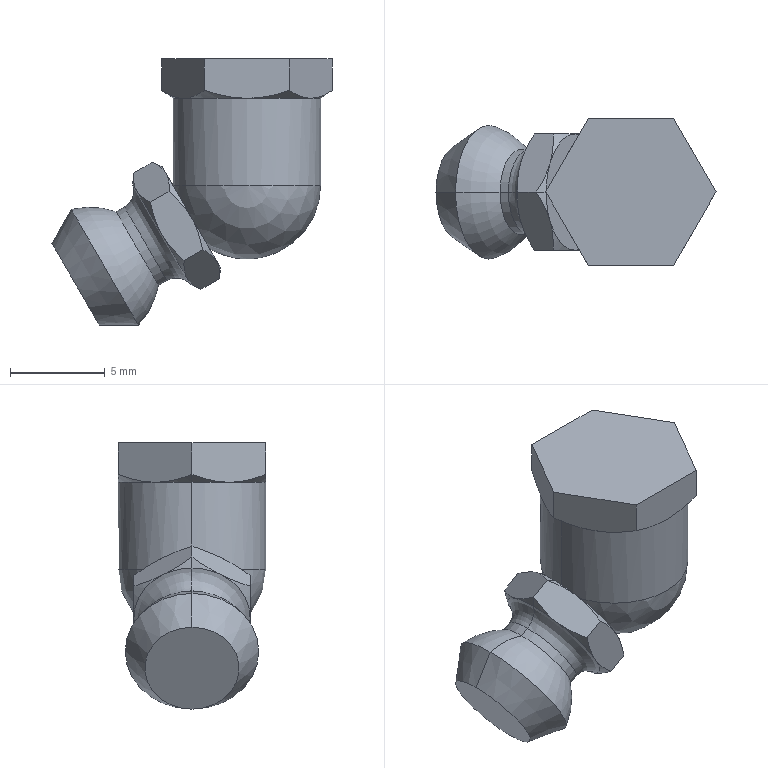Part | STEP file | 2026.6.15-Main Assembly图.sldasm-Part-23 | 1 solid | 51 faces | box 14.821 x 7.8 x 14.088 mm | volume 645.564 mm3 | cone 26 | plane 15 | torus 4 | cylinder 4 | sphere 2 | commonest cylinder face diameters 4.5 x2 7.8 x2